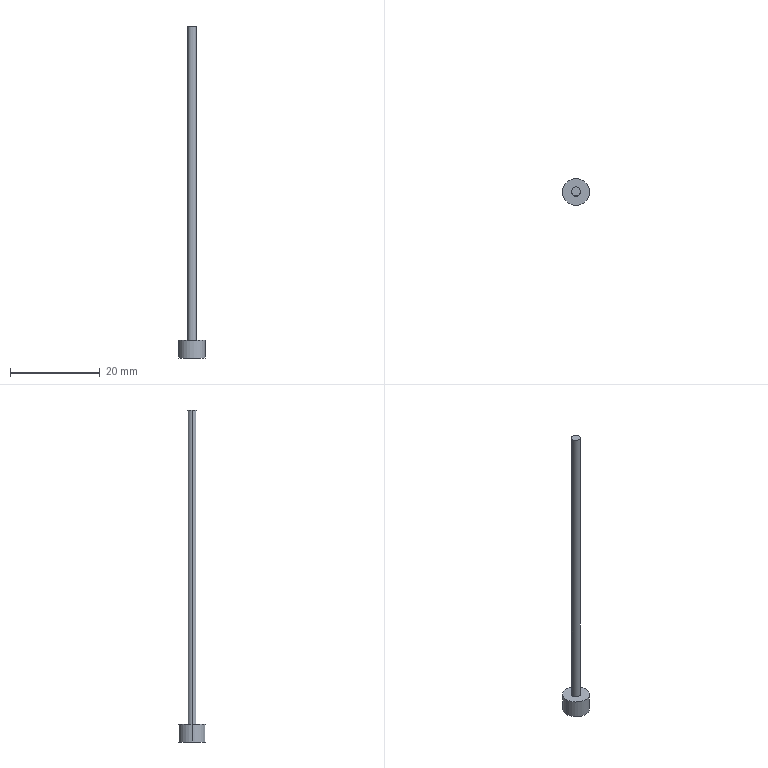Part | Creo | 1 solid | 51 faces | box 6 x 6 x 73.845 mm | volume 331.946 mm3 | other 33 | plane 13 | cylinder 5 | commonest cylinder face diameters 2 x2 6 x2 2.438 x1